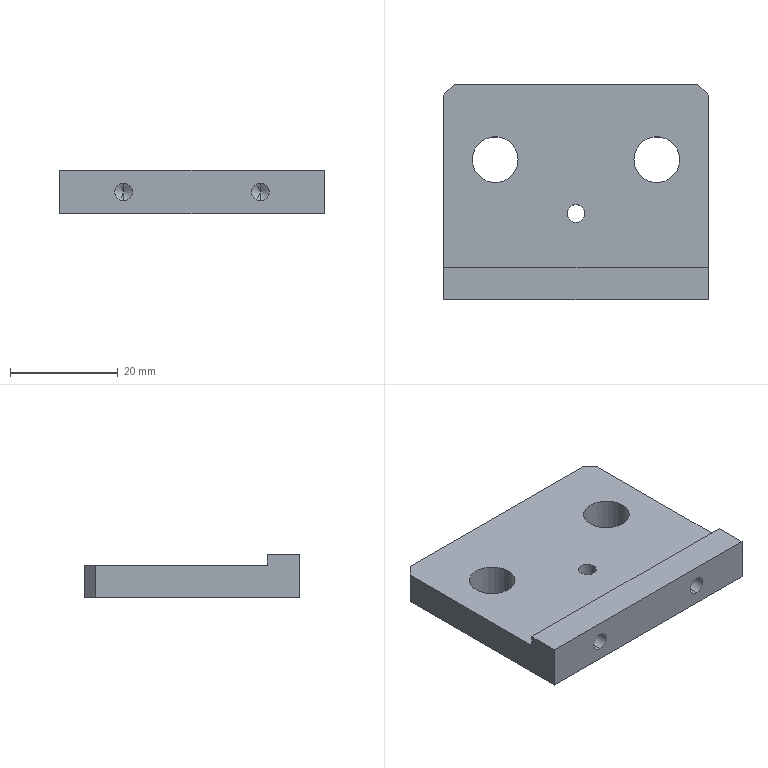Part | SolidWorks | features HoleWzd 2, ICE 2, Chamfer 1, Extrusion 1 | 1 solid | 24 faces | box 49.2 x 40 x 8 mm | volume 11464 mm3 | cylinder 10 | plane 10 | cone 4 | commonest cylinder face diameters 3.3 x6 8.5 x4
STEP:
#1=CARTESIAN_POINT('',(-1.65,-4.,0.));
#2=VERTEX_POINT('',#1);
#3=CARTESIAN_POINT('',(1.65,-4.,0.));
#4=VERTEX_POINT('',#3);
#5=CARTESIAN_POINT('',(0.,-4.,0.));
#6=DIRECTION('',(0.,0.,1.));
#7=DIRECTION('',(1.,0.,0.));
#8=AXIS2_PLACEMENT_3D('',#5,#6,#7);
#9=CIRCLE('',#8,1.65);
#10=EDGE_CURVE('',#2,#4,#9,.T.);
#11=ORIENTED_EDGE('',*,*,#10,.F.);
#12=CARTESIAN_POINT('',(-1.65,-4.,6.));
#13=VERTEX_POINT('',#12);
#14=CARTESIAN_POINT('',(-1.65,-4.,6.));
#15=DIRECTION('',(0.,0.,1.));
#16=VECTOR('',#15,1000.);
#17=LINE('',#14,#16);
#18=EDGE_CURVE('',#2,#13,#17,.T.);
#19=ORIENTED_EDGE('',*,*,#18,.T.);
#20=CARTESIAN_POINT('',(1.65,-4.,6.));
#21=VERTEX_POINT('',#20);
#22=CARTESIAN_POINT('',(0.,-4.,6.));
#23=DIRECTION('',(0.,0.,1.));
#24=DIRECTION('',(1.,0.,0.));
#25=AXIS2_PLACEMENT_3D('',#22,#23,#24);
#26=CIRCLE('',#25,1.65);
#27=EDGE_CURVE('',#13,#21,#26,.T.);
#28=ORIENTED_EDGE('',*,*,#27,.T.);
#29=CARTESIAN_POINT('',(1.65,-4.,6.));
#30=DIRECTION('',(0.,0.,1.));
#31=VECTOR('',#30,1000.);
#32=LINE('',#29,#31);
#33=EDGE_CURVE('',#4,#21,#32,.T.);
#34=ORIENTED_EDGE('',*,*,#33,.F.);
#35=EDGE_LOOP('',(#11,#19,#28,#34));
#36=FACE_OUTER_BOUND('',#35,.T.);
#37=CARTESIAN_POINT('',(0.,-4.,6.));
#38=DIRECTION('',(0.,0.,1.));
#39=DIRECTION('',(1.,0.,0.));
#40=AXIS2_PLACEMENT_3D('',#37,#38,#39);
#41=CYLINDRICAL_SURFACE('',#40,1.65);
#42=ADVANCED_FACE('',(#36),#41,.F.);
#43=CARTESIAN_POINT('',(-19.25,6.,6.));
#44=VERTEX_POINT('',#43);
#45=CARTESIAN_POINT('',(-10.75,6.,6.));
#46=VERTEX_POINT('',#45);
#47=CARTESIAN_POINT('',(-15.,6.,6.));
#48=DIRECTION('',(0.,0.,1.));
#49=DIRECTION('',(1.,0.,0.));
#50=AXIS2_PLACEMENT_3D('',#47,#48,#49);
#51=CIRCLE('',#50,4.25);
#52=EDGE_CURVE('',#44,#46,#51,.T.);
#53=ORIENTED_EDGE('',*,*,#52,.T.);
#54=CARTESIAN_POINT('',(-10.75,6.,0.));
#55=VERTEX_POINT('',#54);
#56=CARTESIAN_POINT('',(-10.75,6.,25.));
#57=DIRECTION('',(0.,0.,-1.));
#58=VECTOR('',#57,1000.);
#59=LINE('',#56,#58);
#60=EDGE_CURVE('',#46,#55,#59,.T.);
#61=ORIENTED_EDGE('',*,*,#60,.T.);
#62=CARTESIAN_POINT('',(-19.25,6.,0.));
#63=VERTEX_POINT('',#62);
#64=CARTESIAN_POINT('',(-15.,6.,0.));
#65=DIRECTION('',(0.,0.,-1.));
#66=DIRECTION('',(-1.,0.,0.));
#67=AXIS2_PLACEMENT_3D('',#64,#65,#66);
#68=CIRCLE('',#67,4.25);
#69=EDGE_CURVE('',#55,#63,#68,.T.);
#70=ORIENTED_EDGE('',*,*,#69,.T.);
#71=CARTESIAN_POINT('',(-19.25,6.,25.));
#72=DIRECTION('',(0.,0.,-1.));
#73=VECTOR('',#72,1000.);
#74=LINE('',#71,#73);
#75=EDGE_CURVE('',#44,#63,#74,.T.);
#76=ORIENTED_EDGE('',*,*,#75,.F.);
#77=EDGE_LOOP('',(#53,#61,#70,#76));
#78=FACE_OUTER_BOUND('',#77,.T.);
#79=CARTESIAN_POINT('',(-15.,6.,25.));
#80=DIRECTION('',(0.,0.,-1.));
#81=DIRECTION('',(-1.,0.,0.));
#82=AXIS2_PLACEMENT_3D('',#79,#80,#81);
#83=CYLINDRICAL_SURFACE('',#82,4.25);
#84=ADVANCED_FACE('',(#78),#83,.F.);
#85=CARTESIAN_POINT('',(10.75,6.,6.));
#86=VERTEX_POINT('',#85);
#87=CARTESIAN_POINT('',(19.25,6.,6.));
#88=VERTEX_POINT('',#87);
#89=CARTESIAN_POINT('',(15.,6.,6.));
#90=DIRECTION('',(0.,0.,1.));
#91=DIRECTION('',(1.,0.,0.));
#92=AXIS2_PLACEMENT_3D('',#89,#90,#91);
#93=CIRCLE('',#92,4.25);
#94=EDGE_CURVE('',#86,#88,#93,.T.);
#95=ORIENTED_EDGE('',*,*,#94,.T.);
#96=CARTESIAN_POINT('',(19.25,6.,0.));
#97=VERTEX_POINT('',#96);
#98=CARTESIAN_POINT('',(19.25,6.,25.));
#99=DIRECTION('',(0.,0.,-1.));
#100=VECTOR('',#99,1000.);
#101=LINE('',#98,#100);
#102=EDGE_CURVE('',#88,#97,#101,.T.);
#103=ORIENTED_EDGE('',*,*,#102,.T.);
#104=CARTESIAN_POINT('',(10.75,6.,0.));
#105=VERTEX_POINT('',#104);
#106=CARTESIAN_POINT('',(15.,6.,0.));
#107=DIRECTION('',(0.,0.,-1.));
#108=DIRECTION('',(-1.,0.,0.));
#109=AXIS2_PLACEMENT_3D('',#106,#107,#108);
#110=CIRCLE('',#109,4.25);
#111=EDGE_CURVE('',#97,#105,#110,.T.);
#112=ORIENTED_EDGE('',*,*,#111,.T.);
#113=CARTESIAN_POINT('',(10.75,6.,25.));
#114=DIRECTION('',(0.,0.,-1.));
#115=VECTOR('',#114,1000.);
#116=LINE('',#113,#115);
#117=EDGE_CURVE('',#86,#105,#116,.T.);
#118=ORIENTED_EDGE('',*,*,#117,.F.);
#119=EDGE_LOOP('',(#95,#103,#112,#118));
#120=FACE_OUTER_BOUND('',#119,.T.);
#121=CARTESIAN_POINT('',(15.,6.,25.));
#122=DIRECTION('',(0.,0.,-1.));
#123=DIRECTION('',(-1.,0.,0.));
#124=AXIS2_PLACEMENT_3D('',#121,#122,#123);
#125=CYLINDRICAL_SURFACE('',#124,4.25);
#126=ADVANCED_FACE('',(#120),#125,.F.);
#127=CARTESIAN_POINT('',(-12.7,-9.9,5.65));
#128=VERTEX_POINT('',#127);
#129=CARTESIAN_POINT('',(-12.7,-9.9,2.35));
#130=VERTEX_POINT('',#129);
#131=CARTESIAN_POINT('',(-12.7,-9.9,4.));
#132=DIRECTION('',(0.,-1.,0.));
#133=DIRECTION('',(0.,0.,-1.));
#134=AXIS2_PLACEMENT_3D('',#131,#132,#133);
#135=CIRCLE('',#134,1.65);
#136=EDGE_CURVE('',#128,#130,#135,.T.);
#137=ORIENTED_EDGE('',*,*,#136,.F.);
#138=CARTESIAN_POINT('',(-12.7,-20.,5.65));
#139=VERTEX_POINT('',#138);
#140=CARTESIAN_POINT('',(-12.7,-20.,5.65));
#141=DIRECTION('',(0.,-1.,0.));
#142=VECTOR('',#141,1000.);
#143=LINE('',#140,#142);
#144=EDGE_CURVE('',#128,#139,#143,.T.);
#145=ORIENTED_EDGE('',*,*,#144,.T.);
#146=CARTESIAN_POINT('',(-12.7,-20.,2.35));
#147=VERTEX_POINT('',#146);
#148=CARTESIAN_POINT('',(-12.7,-20.,4.));
#149=DIRECTION('',(0.,-1.,0.));
#150=DIRECTION('',(0.,0.,-1.));
#151=AXIS2_PLACEMENT_3D('',#148,#149,#150);
#152=CIRCLE('',#151,1.65);
#153=EDGE_CURVE('',#139,#147,#152,.T.);
#154=ORIENTED_EDGE('',*,*,#153,.T.);
#155=CARTESIAN_POINT('',(-12.7,-20.,2.35));
#156=DIRECTION('',(0.,-1.,0.));
#157=VECTOR('',#156,1000.);
#158=LINE('',#155,#157);
#159=EDGE_CURVE('',#130,#147,#158,.T.);
#160=ORIENTED_EDGE('',*,*,#159,.F.);
#161=EDGE_LOOP('',(#137,#145,#154,#160));
#162=FACE_OUTER_BOUND('',#161,.T.);
#163=CARTESIAN_POINT('',(-12.7,-20.,4.));
#164=DIRECTION('',(0.,-1.,0.));
#165=DIRECTION('',(0.,0.,-1.));
#166=AXIS2_PLACEMENT_3D('',#163,#164,#165);
#167=CYLINDRICAL_SURFACE('',#166,1.65);
#168=ADVANCED_FACE('',(#162),#167,.F.);
#169=CARTESIAN_POINT('',(-12.7,-8.909,4.));
#170=VERTEX_POINT('',#169);
#171=CARTESIAN_POINT('',(-12.7,-9.9,2.35));
#172=DIRECTION('',(0.,-0.515,-0.8572));
#173=VECTOR('',#172,1000.);
#174=LINE('',#171,#173);
#175=EDGE_CURVE('',#170,#130,#174,.T.);
#176=ORIENTED_EDGE('',*,*,#175,.F.);
#177=CARTESIAN_POINT('',(-12.7,-9.9,5.65));
#178=DIRECTION('',(0.,-0.515,0.8572));
#179=VECTOR('',#178,1000.);
#180=LINE('',#177,#179);
#181=EDGE_CURVE('',#170,#128,#180,.T.);
#182=ORIENTED_EDGE('',*,*,#181,.T.);
#183=ORIENTED_EDGE('',*,*,#136,.T.);
#184=EDGE_LOOP('',(#176,#182,#183));
#185=FACE_OUTER_BOUND('',#184,.T.);
#186=CARTESIAN_POINT('',(-12.7,-9.9,4.));
#187=DIRECTION('',(0.,-1.,0.));
#188=DIRECTION('',(0.,0.,-1.));
#189=AXIS2_PLACEMENT_3D('',#186,#187,#188);
#190=CONICAL_SURFACE('',#189,1.65,1.03);
#191=ADVANCED_FACE('',(#185),#190,.F.);
#192=CARTESIAN_POINT('',(12.7,-9.9,5.65));
#193=VERTEX_POINT('',#192);
#194=CARTESIAN_POINT('',(12.7,-9.9,2.35));
#195=VERTEX_POINT('',#194);
#196=CARTESIAN_POINT('',(12.7,-9.9,4.));
#197=DIRECTION('',(0.,-1.,0.));
#198=DIRECTION('',(0.,0.,-1.));
#199=AXIS2_PLACEMENT_3D('',#196,#197,#198);
#200=CIRCLE('',#199,1.65);
#201=EDGE_CURVE('',#193,#195,#200,.T.);
#202=ORIENTED_EDGE('',*,*,#201,.F.);
#203=CARTESIAN_POINT('',(12.7,-20.,5.65));
#204=VERTEX_POINT('',#203);
#205=CARTESIAN_POINT('',(12.7,-20.,5.65));
#206=DIRECTION('',(0.,-1.,0.));
#207=VECTOR('',#206,1000.);
#208=LINE('',#205,#207);
#209=EDGE_CURVE('',#193,#204,#208,.T.);
#210=ORIENTED_EDGE('',*,*,#209,.T.);
#211=CARTESIAN_POINT('',(12.7,-20.,2.35));
#212=VERTEX_POINT('',#211);
#213=CARTESIAN_POINT('',(12.7,-20.,4.));
#214=DIRECTION('',(0.,-1.,0.));
#215=DIRECTION('',(0.,0.,-1.));
#216=AXIS2_PLACEMENT_3D('',#213,#214,#215);
#217=CIRCLE('',#216,1.65);
#218=EDGE_CURVE('',#204,#212,#217,.T.);
#219=ORIENTED_EDGE('',*,*,#218,.T.);
#220=CARTESIAN_POINT('',(12.7,-20.,2.35));
#221=DIRECTION('',(0.,-1.,0.));
#222=VECTOR('',#221,1000.);
#223=LINE('',#220,#222);
#224=EDGE_CURVE('',#195,#212,#223,.T.);
#225=ORIENTED_EDGE('',*,*,#224,.F.);
#226=EDGE_LOOP('',(#202,#210,#219,#225));
#227=FACE_OUTER_BOUND('',#226,.T.);
#228=CARTESIAN_POINT('',(12.7,-20.,4.));
#229=DIRECTION('',(0.,-1.,0.));
#230=DIRECTION('',(0.,0.,-1.));
#231=AXIS2_PLACEMENT_3D('',#228,#229,#230);
#232=CYLINDRICAL_SURFACE('',#231,1.65);
#233=ADVANCED_FACE('',(#227),#232,.F.);
#234=CARTESIAN_POINT('',(12.7,-8.909,4.));
#235=VERTEX_POINT('',#234);
#236=CARTESIAN_POINT('',(12.7,-9.9,2.35));
#237=DIRECTION('',(0.,-0.515,-0.8572));
#238=VECTOR('',#237,1000.);
#239=LINE('',#236,#238);
#240=EDGE_CURVE('',#235,#195,#239,.T.);
#241=ORIENTED_EDGE('',*,*,#240,.F.);
#242=CARTESIAN_POINT('',(12.7,-9.9,5.65));
#243=DIRECTION('',(0.,-0.515,0.8572));
#244=VECTOR('',#243,1000.);
#245=LINE('',#242,#244);
#246=EDGE_CURVE('',#235,#193,#245,.T.);
#247=ORIENTED_EDGE('',*,*,#246,.T.);
#248=ORIENTED_EDGE('',*,*,#201,.T.);
#249=EDGE_LOOP('',(#241,#247,#248));
#250=FACE_OUTER_BOUND('',#249,.T.);
#251=CARTESIAN_POINT('',(12.7,-9.9,4.));
#252=DIRECTION('',(0.,-1.,0.));
#253=DIRECTION('',(0.,0.,-1.));
#254=AXIS2_PLACEMENT_3D('',#251,#252,#253);
#255=CONICAL_SURFACE('',#254,1.65,1.03);
#256=ADVANCED_FACE('',(#250),#255,.F.);
#257=CARTESIAN_POINT('',(22.6,20.,6.));
#258=VERTEX_POINT('',#257);
#259=CARTESIAN_POINT('',(-22.6,20.,6.));
#260=VERTEX_POINT('',#259);
#261=CARTESIAN_POINT('',(-24.6,20.,6.));
#262=DIRECTION('',(-1.,0.,0.));
#263=VECTOR('',#262,1000.);
#264=LINE('',#261,#263);
#265=EDGE_CURVE('',#258,#260,#264,.T.);
#266=ORIENTED_EDGE('',*,*,#265,.F.);
#267=CARTESIAN_POINT('',(22.6,20.,0.));
#268=VERTEX_POINT('',#267);
#269=CARTESIAN_POINT('',(22.6,20.,8.));
#270=DIRECTION('',(0.,0.,-1.));
#271=VECTOR('',#270,1000.);
#272=LINE('',#269,#271);
#273=EDGE_CURVE('',#258,#268,#272,.T.);
#274=ORIENTED_EDGE('',*,*,#273,.T.);
#275=CARTESIAN_POINT('',(-22.6,20.,0.));
#276=VERTEX_POINT('',#275);
#277=CARTESIAN_POINT('',(-24.6,20.,0.));
#278=DIRECTION('',(-1.,0.,0.));
#279=VECTOR('',#278,1000.);
#280=LINE('',#277,#279);
#281=EDGE_CURVE('',#268,#276,#280,.T.);
#282=ORIENTED_EDGE('',*,*,#281,.T.);
#283=CARTESIAN_POINT('',(-22.6,20.,8.));
#284=DIRECTION('',(0.,0.,1.));
#285=VECTOR('',#284,1000.);
#286=LINE('',#283,#285);
#287=EDGE_CURVE('',#276,#260,#286,.T.);
#288=ORIENTED_EDGE('',*,*,#287,.T.);
#289=EDGE_LOOP('',(#266,#274,#282,#288));
#290=FACE_OUTER_BOUND('',#289,.T.);
#291=CARTESIAN_POINT('',(-24.6,20.,8.));
#292=DIRECTION('',(0.,-1.,0.));
#293=DIRECTION('',(0.,0.,-1.));
#294=AXIS2_PLACEMENT_3D('',#291,#292,#293);
#295=PLANE('',#294);
#296=ADVANCED_FACE('',(#290),#295,.F.);
#297=ORIENTED_EDGE('',*,*,#273,.F.);
#298=CARTESIAN_POINT('',(24.6,18.,6.));
#299=VERTEX_POINT('',#298);
#300=CARTESIAN_POINT('',(22.6,20.,6.));
#301=DIRECTION('',(0.7071,-0.7071,0.));
#302=VECTOR('',#301,1000.);
#303=LINE('',#300,#302);
#304=EDGE_CURVE('',#258,#299,#303,.T.);
#305=ORIENTED_EDGE('',*,*,#304,.T.);
#306=CARTESIAN_POINT('',(24.6,18.,0.));
#307=VERTEX_POINT('',#306);
#308=CARTESIAN_POINT('',(24.6,18.,8.));
#309=DIRECTION('',(0.,0.,1.));
#310=VECTOR('',#309,1000.);
#311=LINE('',#308,#310);
#312=EDGE_CURVE('',#307,#299,#311,.T.);
#313=ORIENTED_EDGE('',*,*,#312,.F.);
#314=CARTESIAN_POINT('',(22.6,20.,0.));
#315=DIRECTION('',(0.7071,-0.7071,0.));
#316=VECTOR('',#315,1000.);
#317=LINE('',#314,#316);
#318=EDGE_CURVE('',#268,#307,#317,.T.);
#319=ORIENTED_EDGE('',*,*,#318,.F.);
#320=EDGE_LOOP('',(#297,#305,#313,#319));
#321=FACE_OUTER_BOUND('',#320,.T.);
#322=CARTESIAN_POINT('',(22.6,20.,8.));
#323=DIRECTION('',(-0.7071,-0.7071,0.));
#324=DIRECTION('',(0.,0.,-1.));
#325=AXIS2_PLACEMENT_3D('',#322,#323,#324);
#326=PLANE('',#325);
#327=ADVANCED_FACE('',(#321),#326,.F.);
#328=CARTESIAN_POINT('',(-24.6,18.,6.));
#329=VERTEX_POINT('',#328);
#330=CARTESIAN_POINT('',(-24.6,18.,0.));
#331=VERTEX_POINT('',#330);
#332=CARTESIAN_POINT('',(-24.6,18.,8.));
#333=DIRECTION('',(0.,0.,-1.));
#334=VECTOR('',#333,1000.);
#335=LINE('',#332,#334);
#336=EDGE_CURVE('',#329,#331,#335,.T.);
#337=ORIENTED_EDGE('',*,*,#336,.F.);
#338=CARTESIAN_POINT('',(-24.6,18.,6.));
#339=DIRECTION('',(0.7071,0.7071,0.));
#340=VECTOR('',#339,1000.);
#341=LINE('',#338,#340);
#342=EDGE_CURVE('',#329,#260,#341,.T.);
#343=ORIENTED_EDGE('',*,*,#342,.T.);
#344=ORIENTED_EDGE('',*,*,#287,.F.);
#345=CARTESIAN_POINT('',(-24.6,18.,0.));
#346=DIRECTION('',(0.7071,0.7071,0.));
#347=VECTOR('',#346,1000.);
#348=LINE('',#345,#347);
#349=EDGE_CURVE('',#331,#276,#348,.T.);
#350=ORIENTED_EDGE('',*,*,#349,.F.);
#351=EDGE_LOOP('',(#337,#343,#344,#350));
#352=FACE_OUTER_BOUND('',#351,.T.);
#353=CARTESIAN_POINT('',(-24.6,18.,8.));
#354=DIRECTION('',(0.7071,-0.7071,0.));
#355=DIRECTION('',(0.,0.,-1.));
#356=AXIS2_PLACEMENT_3D('',#353,#354,#355);
#357=PLANE('',#356);
#358=ADVANCED_FACE('',(#352),#357,.F.);
#359=CARTESIAN_POINT('',(24.6,-14.,6.));
#360=VERTEX_POINT('',#359);
#361=CARTESIAN_POINT('',(24.6,20.,6.));
#362=DIRECTION('',(0.,1.,0.));
#363=VECTOR('',#362,1000.);
#364=LINE('',#361,#363);
#365=EDGE_CURVE('',#360,#299,#364,.T.);
#366=ORIENTED_EDGE('',*,*,#365,.F.);
#367=CARTESIAN_POINT('',(24.6,-14.,8.));
#368=VERTEX_POINT('',#367);
#369=CARTESIAN_POINT('',(24.6,-14.,8.));
#370=DIRECTION('',(0.,0.,1.));
#371=VECTOR('',#370,1000.);
#372=LINE('',#369,#371);
#373=EDGE_CURVE('',#360,#368,#372,.T.);
#374=ORIENTED_EDGE('',*,*,#373,.T.);
#375=CARTESIAN_POINT('',(24.6,-20.,8.));
#376=VERTEX_POINT('',#375);
#377=CARTESIAN_POINT('',(24.6,20.,8.));
#378=DIRECTION('',(0.,1.,0.));
#379=VECTOR('',#378,1000.);
#380=LINE('',#377,#379);
#381=EDGE_CURVE('',#376,#368,#380,.T.);
#382=ORIENTED_EDGE('',*,*,#381,.F.);
#383=CARTESIAN_POINT('',(24.6,-20.,0.));
#384=VERTEX_POINT('',#383);
#385=CARTESIAN_POINT('',(24.6,-20.,8.));
#386=DIRECTION('',(0.,0.,-1.));
#387=VECTOR('',#386,1000.);
#388=LINE('',#385,#387);
#389=EDGE_CURVE('',#376,#384,#388,.T.);
#390=ORIENTED_EDGE('',*,*,#389,.T.);
#391=CARTESIAN_POINT('',(24.6,20.,0.));
#392=DIRECTION('',(0.,1.,0.));
#393=VECTOR('',#392,1000.);
#394=LINE('',#391,#393);
#395=EDGE_CURVE('',#384,#307,#394,.T.);
#396=ORIENTED_EDGE('',*,*,#395,.T.);
#397=ORIENTED_EDGE('',*,*,#312,.T.);
#398=EDGE_LOOP('',(#366,#374,#382,#390,#396,#397));
#399=FACE_OUTER_BOUND('',#398,.T.);
#400=CARTESIAN_POINT('',(24.6,20.,8.));
#401=DIRECTION('',(-1.,0.,0.));
#402=DIRECTION('',(0.,-1.,0.));
#403=AXIS2_PLACEMENT_3D('',#400,#401,#402);
#404=PLANE('',#403);
#405=ADVANCED_FACE('',(#399),#404,.F.);
#406=CARTESIAN_POINT('',(-24.6,-14.,8.));
#407=VERTEX_POINT('',#406);
#408=CARTESIAN_POINT('',(-24.6,-20.,8.));
#409=VERTEX_POINT('',#408);
#410=CARTESIAN_POINT('',(-24.6,20.,8.));
#411=DIRECTION('',(0.,-1.,0.));
#412=VECTOR('',#411,1000.);
#413=LINE('',#410,#412);
#414=EDGE_CURVE('',#407,#409,#413,.T.);
#415=ORIENTED_EDGE('',*,*,#414,.F.);
#416=CARTESIAN_POINT('',(-24.6,-14.,6.));
#417=VERTEX_POINT('',#416);
#418=CARTESIAN_POINT('',(-24.6,-14.,8.));
#419=DIRECTION('',(0.,0.,-1.));
#420=VECTOR('',#419,1000.);
#421=LINE('',#418,#420);
#422=EDGE_CURVE('',#407,#417,#421,.T.);
#423=ORIENTED_EDGE('',*,*,#422,.T.);
#424=CARTESIAN_POINT('',(-24.6,20.,6.));
#425=DIRECTION('',(0.,-1.,0.));
#426=VECTOR('',#425,1000.);
#427=LINE('',#424,#426);
#428=EDGE_CURVE('',#329,#417,#427,.T.);
#429=ORIENTED_EDGE('',*,*,#428,.F.);
#430=ORIENTED_EDGE('',*,*,#336,.T.);
#431=CARTESIAN_POINT('',(-24.6,-20.,0.));
#432=VERTEX_POINT('',#431);
#433=CARTESIAN_POINT('',(-24.6,20.,0.));
#434=DIRECTION('',(0.,-1.,0.));
#435=VECTOR('',#434,1000.);
#436=LINE('',#433,#435);
#437=EDGE_CURVE('',#331,#432,#436,.T.);
#438=ORIENTED_EDGE('',*,*,#437,.T.);
#439=CARTESIAN_POINT('',(-24.6,-20.,8.));
#440=DIRECTION('',(0.,0.,-1.));
#441=VECTOR('',#440,1000.);
#442=LINE('',#439,#441);
#443=EDGE_CURVE('',#409,#432,#442,.T.);
#444=ORIENTED_EDGE('',*,*,#443,.F.);
#445=EDGE_LOOP('',(#415,#423,#429,#430,#438,#444));
#446=FACE_OUTER_BOUND('',#445,.T.);
#447=CARTESIAN_POINT('',(-24.6,20.,8.));
#448=DIRECTION('',(1.,0.,0.));
#449=DIRECTION('',(0.,1.,0.));
#450=AXIS2_PLACEMENT_3D('',#447,#448,#449);
#451=PLANE('',#450);
#452=ADVANCED_FACE('',(#446),#451,.F.);
#453=CARTESIAN_POINT('',(-12.7,-20.,4.));
#454=DIRECTION('',(0.,-1.,0.));
#455=DIRECTION('',(0.,0.,-1.));
#456=AXIS2_PLACEMENT_3D('',#453,#454,#455);
#457=CIRCLE('',#456,1.65);
#458=EDGE_CURVE('',#147,#139,#457,.T.);
#459=ORIENTED_EDGE('',*,*,#458,.F.);
#460=ORIENTED_EDGE('',*,*,#153,.F.);
#461=EDGE_LOOP('',(#459,#460));
#462=FACE_BOUND('',#461,.T.);
#463=CARTESIAN_POINT('',(12.7,-20.,4.));
#464=DIRECTION('',(0.,-1.,0.));
#465=DIRECTION('',(0.,0.,-1.));
#466=AXIS2_PLACEMENT_3D('',#463,#464,#465);
#467=CIRCLE('',#466,1.65);
#468=EDGE_CURVE('',#212,#204,#467,.T.);
#469=ORIENTED_EDGE('',*,*,#468,.F.);
#470=ORIENTED_EDGE('',*,*,#218,.F.);
#471=EDGE_LOOP('',(#469,#470));
#472=FACE_BOUND('',#471,.T.);
#473=CARTESIAN_POINT('',(-24.6,-20.,0.));
#474=DIRECTION('',(1.,0.,0.));
#475=VECTOR('',#474,1000.);
#476=LINE('',#473,#475);
#477=EDGE_CURVE('',#432,#384,#476,.T.);
#478=ORIENTED_EDGE('',*,*,#477,.T.);
#479=ORIENTED_EDGE('',*,*,#389,.F.);
#480=CARTESIAN_POINT('',(-24.6,-20.,8.));
#481=DIRECTION('',(1.,0.,0.));
#482=VECTOR('',#481,1000.);
#483=LINE('',#480,#482);
#484=EDGE_CURVE('',#409,#376,#483,.T.);
#485=ORIENTED_EDGE('',*,*,#484,.F.);
#486=ORIENTED_EDGE('',*,*,#443,.T.);
#487=EDGE_LOOP('',(#478,#479,#485,#486));
#488=FACE_OUTER_BOUND('',#487,.T.);
#489=CARTESIAN_POINT('',(-24.6,-20.,8.));
#490=DIRECTION('',(0.,1.,0.));
#491=DIRECTION('',(0.,0.,1.));
#492=AXIS2_PLACEMENT_3D('',#489,#490,#491);
#493=PLANE('',#492);
#494=ADVANCED_FACE('',(#462,#472,#488),#493,.F.);
#495=CARTESIAN_POINT('',(-24.969,-14.,8.));
#496=DIRECTION('',(1.,0.,0.));
#497=VECTOR('',#496,1000.);
#498=LINE('',#495,#497);
#499=EDGE_CURVE('',#407,#368,#498,.T.);
#500=ORIENTED_EDGE('',*,*,#499,.F.);
#501=ORIENTED_EDGE('',*,*,#414,.T.);
#502=ORIENTED_EDGE('',*,*,#484,.T.);
#503=ORIENTED_EDGE('',*,*,#381,.T.);
#504=EDGE_LOOP('',(#500,#501,#502,#503));
#505=FACE_OUTER_BOUND('',#504,.T.);
#506=CARTESIAN_POINT('',(0.,0.,8.));
#507=DIRECTION('',(0.,0.,1.));
#508=DIRECTION('',(1.,0.,0.));
#509=AXIS2_PLACEMENT_3D('',#506,#507,#508);
#510=PLANE('',#509);
#511=ADVANCED_FACE('',(#505),#510,.T.);
#512=CARTESIAN_POINT('',(0.,-4.,0.));
#513=DIRECTION('',(0.,0.,1.));
#514=DIRECTION('',(1.,0.,0.));
#515=AXIS2_PLACEMENT_3D('',#512,#513,#514);
#516=CIRCLE('',#515,1.65);
#517=EDGE_CURVE('',#4,#2,#516,.T.);
#518=ORIENTED_EDGE('',*,*,#517,.T.);
#519=ORIENTED_EDGE('',*,*,#10,.T.);
#520=EDGE_LOOP('',(#518,#519));
#521=FACE_BOUND('',#520,.T.);
#522=CARTESIAN_POINT('',(-15.,6.,0.));
#523=DIRECTION('',(0.,0.,-1.));
#524=DIRECTION('',(-1.,0.,0.));
#525=AXIS2_PLACEMENT_3D('',#522,#523,#524);
#526=CIRCLE('',#525,4.25);
#527=EDGE_CURVE('',#63,#55,#526,.T.);
#528=ORIENTED_EDGE('',*,*,#527,.F.);
#529=ORIENTED_EDGE('',*,*,#69,.F.);
#530=EDGE_LOOP('',(#528,#529));
#531=FACE_BOUND('',#530,.T.);
#532=CARTESIAN_POINT('',(15.,6.,0.));
#533=DIRECTION('',(0.,0.,-1.));
#534=DIRECTION('',(-1.,0.,0.));
#535=AXIS2_PLACEMENT_3D('',#532,#533,#534);
#536=CIRCLE('',#535,4.25);
#537=EDGE_CURVE('',#105,#97,#536,.T.);
#538=ORIENTED_EDGE('',*,*,#537,.F.);
#539=ORIENTED_EDGE('',*,*,#111,.F.);
#540=EDGE_LOOP('',(#538,#539));
#541=FACE_BOUND('',#540,.T.);
#542=ORIENTED_EDGE('',*,*,#281,.F.);
#543=ORIENTED_EDGE('',*,*,#318,.T.);
#544=ORIENTED_EDGE('',*,*,#395,.F.);
#545=ORIENTED_EDGE('',*,*,#477,.F.);
#546=ORIENTED_EDGE('',*,*,#437,.F.);
#547=ORIENTED_EDGE('',*,*,#349,.T.);
#548=EDGE_LOOP('',(#542,#543,#544,#545,#546,#547));
#549=FACE_OUTER_BOUND('',#548,.T.);
#550=CARTESIAN_POINT('',(0.,0.,0.));
#551=DIRECTION('',(0.,0.,1.));
#552=DIRECTION('',(1.,0.,0.));
#553=AXIS2_PLACEMENT_3D('',#550,#551,#552);
#554=PLANE('',#553);
#555=ADVANCED_FACE('',(#521,#531,#541,#549),#554,.F.);
#556=ORIENTED_EDGE('',*,*,#246,.F.);
#557=ORIENTED_EDGE('',*,*,#240,.T.);
#558=CARTESIAN_POINT('',(12.7,-9.9,4.));
#559=DIRECTION('',(0.,-1.,0.));
#560=DIRECTION('',(0.,0.,-1.));
#561=AXIS2_PLACEMENT_3D('',#558,#559,#560);
#562=CIRCLE('',#561,1.65);
#563=EDGE_CURVE('',#195,#193,#562,.T.);
#564=ORIENTED_EDGE('',*,*,#563,.T.);
#565=EDGE_LOOP('',(#556,#557,#564));
#566=FACE_OUTER_BOUND('',#565,.T.);
#567=CARTESIAN_POINT('',(12.7,-9.9,4.));
#568=DIRECTION('',(0.,-1.,0.));
#569=DIRECTION('',(0.,0.,-1.));
#570=AXIS2_PLACEMENT_3D('',#567,#568,#569);
#571=CONICAL_SURFACE('',#570,1.65,1.03);
#572=ADVANCED_FACE('',(#566),#571,.F.);
#573=ORIENTED_EDGE('',*,*,#209,.F.);
#574=ORIENTED_EDGE('',*,*,#563,.F.);
#575=ORIENTED_EDGE('',*,*,#224,.T.);
#576=ORIENTED_EDGE('',*,*,#468,.T.);
#577=EDGE_LOOP('',(#573,#574,#575,#576));
#578=FACE_OUTER_BOUND('',#577,.T.);
#579=CARTESIAN_POINT('',(12.7,-20.,4.));
#580=DIRECTION('',(0.,-1.,0.));
#581=DIRECTION('',(0.,0.,-1.));
#582=AXIS2_PLACEMENT_3D('',#579,#580,#581);
#583=CYLINDRICAL_SURFACE('',#582,1.65);
#584=ADVANCED_FACE('',(#578),#583,.F.);
#585=ORIENTED_EDGE('',*,*,#181,.F.);
#586=ORIENTED_EDGE('',*,*,#175,.T.);
#587=CARTESIAN_POINT('',(-12.7,-9.9,4.));
#588=DIRECTION('',(0.,-1.,0.));
#589=DIRECTION('',(0.,0.,-1.));
#590=AXIS2_PLACEMENT_3D('',#587,#588,#589);
#591=CIRCLE('',#590,1.65);
#592=EDGE_CURVE('',#130,#128,#591,.T.);
#593=ORIENTED_EDGE('',*,*,#592,.T.);
#594=EDGE_LOOP('',(#585,#586,#593));
#595=FACE_OUTER_BOUND('',#594,.T.);
#596=CARTESIAN_POINT('',(-12.7,-9.9,4.));
#597=DIRECTION('',(0.,-1.,0.));
#598=DIRECTION('',(0.,0.,-1.));
#599=AXIS2_PLACEMENT_3D('',#596,#597,#598);
#600=CONICAL_SURFACE('',#599,1.65,1.03);
#601=ADVANCED_FACE('',(#595),#600,.F.);
#602=ORIENTED_EDGE('',*,*,#144,.F.);
#603=ORIENTED_EDGE('',*,*,#592,.F.);
#604=ORIENTED_EDGE('',*,*,#159,.T.);
#605=ORIENTED_EDGE('',*,*,#458,.T.);
#606=EDGE_LOOP('',(#602,#603,#604,#605));
#607=FACE_OUTER_BOUND('',#606,.T.);
#608=CARTESIAN_POINT('',(-12.7,-20.,4.));
#609=DIRECTION('',(0.,-1.,0.));
#610=DIRECTION('',(0.,0.,-1.));
#611=AXIS2_PLACEMENT_3D('',#608,#609,#610);
#612=CYLINDRICAL_SURFACE('',#611,1.65);
#613=ADVANCED_FACE('',(#607),#612,.F.);
#614=CARTESIAN_POINT('',(-24.969,-14.,6.));
#615=DIRECTION('',(1.,0.,0.));
#616=VECTOR('',#615,1000.);
#617=LINE('',#614,#616);
#618=EDGE_CURVE('',#417,#360,#617,.T.);
#619=ORIENTED_EDGE('',*,*,#618,.F.);
#620=ORIENTED_EDGE('',*,*,#422,.F.);
#621=ORIENTED_EDGE('',*,*,#499,.T.);
#622=ORIENTED_EDGE('',*,*,#373,.F.);
#623=EDGE_LOOP('',(#619,#620,#621,#622));
#624=FACE_OUTER_BOUND('',#623,.T.);
#625=CARTESIAN_POINT('',(-24.969,-14.,6.));
#626=DIRECTION('',(0.,-1.,0.));
#627=DIRECTION('',(0.,0.,-1.));
#628=AXIS2_PLACEMENT_3D('',#625,#626,#627);
#629=PLANE('',#628);
#630=ADVANCED_FACE('',(#624),#629,.F.);
#631=CARTESIAN_POINT('',(0.,-4.,6.));
#632=DIRECTION('',(0.,0.,1.));
#633=DIRECTION('',(1.,0.,0.));
#634=AXIS2_PLACEMENT_3D('',#631,#632,#633);
#635=CIRCLE('',#634,1.65);
#636=EDGE_CURVE('',#21,#13,#635,.T.);
#637=ORIENTED_EDGE('',*,*,#636,.F.);
#638=ORIENTED_EDGE('',*,*,#27,.F.);
#639=EDGE_LOOP('',(#637,#638));
#640=FACE_BOUND('',#639,.T.);
#641=ORIENTED_EDGE('',*,*,#52,.F.);
#642=CARTESIAN_POINT('',(-15.,6.,6.));
#643=DIRECTION('',(0.,0.,1.));
#644=DIRECTION('',(1.,0.,0.));
#645=AXIS2_PLACEMENT_3D('',#642,#643,#644);
#646=CIRCLE('',#645,4.25);
#647=EDGE_CURVE('',#46,#44,#646,.T.);
#648=ORIENTED_EDGE('',*,*,#647,.F.);
#649=EDGE_LOOP('',(#641,#648));
#650=FACE_BOUND('',#649,.T.);
#651=ORIENTED_EDGE('',*,*,#94,.F.);
#652=CARTESIAN_POINT('',(15.,6.,6.));
#653=DIRECTION('',(0.,0.,1.));
#654=DIRECTION('',(1.,0.,0.));
#655=AXIS2_PLACEMENT_3D('',#652,#653,#654);
#656=CIRCLE('',#655,4.25);
#657=EDGE_CURVE('',#88,#86,#656,.T.);
#658=ORIENTED_EDGE('',*,*,#657,.F.);
#659=EDGE_LOOP('',(#651,#658));
#660=FACE_BOUND('',#659,.T.);
#661=ORIENTED_EDGE('',*,*,#365,.T.);
#662=ORIENTED_EDGE('',*,*,#304,.F.);
#663=ORIENTED_EDGE('',*,*,#265,.T.);
#664=ORIENTED_EDGE('',*,*,#342,.F.);
#665=ORIENTED_EDGE('',*,*,#428,.T.);
#666=ORIENTED_EDGE('',*,*,#618,.T.);
#667=EDGE_LOOP('',(#661,#662,#663,#664,#665,#666));
#668=FACE_OUTER_BOUND('',#667,.T.);
#669=CARTESIAN_POINT('',(0.,0.,6.));
#670=DIRECTION('',(0.,0.,1.));
#671=DIRECTION('',(1.,0.,0.));
#672=AXIS2_PLACEMENT_3D('',#669,#670,#671);
#673=PLANE('',#672);
#674=ADVANCED_FACE('',(#640,#650,#660,#668),#673,.T.);
#675=ORIENTED_EDGE('',*,*,#102,.F.);
#676=ORIENTED_EDGE('',*,*,#657,.T.);
#677=ORIENTED_EDGE('',*,*,#117,.T.);
#678=ORIENTED_EDGE('',*,*,#537,.T.);
#679=EDGE_LOOP('',(#675,#676,#677,#678));
#680=FACE_OUTER_BOUND('',#679,.T.);
#681=CARTESIAN_POINT('',(15.,6.,25.));
#682=DIRECTION('',(0.,0.,-1.));
#683=DIRECTION('',(-1.,0.,0.));
#684=AXIS2_PLACEMENT_3D('',#681,#682,#683);
#685=CYLINDRICAL_SURFACE('',#684,4.25);
#686=ADVANCED_FACE('',(#680),#685,.F.);
#687=ORIENTED_EDGE('',*,*,#60,.F.);
#688=ORIENTED_EDGE('',*,*,#647,.T.);
#689=ORIENTED_EDGE('',*,*,#75,.T.);
#690=ORIENTED_EDGE('',*,*,#527,.T.);
#691=EDGE_LOOP('',(#687,#688,#689,#690));
#692=FACE_OUTER_BOUND('',#691,.T.);
#693=CARTESIAN_POINT('',(-15.,6.,25.));
#694=DIRECTION('',(0.,0.,-1.));
#695=DIRECTION('',(-1.,0.,0.));
#696=AXIS2_PLACEMENT_3D('',#693,#694,#695);
#697=CYLINDRICAL_SURFACE('',#696,4.25);
#698=ADVANCED_FACE('',(#692),#697,.F.);
#699=ORIENTED_EDGE('',*,*,#18,.F.);
#700=ORIENTED_EDGE('',*,*,#517,.F.);
#701=ORIENTED_EDGE('',*,*,#33,.T.);
#702=ORIENTED_EDGE('',*,*,#636,.T.);
#703=EDGE_LOOP('',(#699,#700,#701,#702));
#704=FACE_OUTER_BOUND('',#703,.T.);
#705=CARTESIAN_POINT('',(0.,-4.,6.));
#706=DIRECTION('',(0.,0.,1.));
#707=DIRECTION('',(1.,0.,0.));
#708=AXIS2_PLACEMENT_3D('',#705,#706,#707);
#709=CYLINDRICAL_SURFACE('',#708,1.65);
#710=ADVANCED_FACE('',(#704),#709,.F.);
#711=CLOSED_SHELL('',(#42,#84,#126,#168,#191,#233,#256,#296,#327,#358,#405,#452,#494,#511,#555,#572,#584,#601,#613,#630,#674,#686,#698,#710));
#712=MANIFOLD_SOLID_BREP('',#711);
#713=CARTESIAN_POINT('',(0.,0.,0.));
#714=DIRECTION('',(0.,0.,1.));
#715=DIRECTION('',(1.,0.,0.));
#716=AXIS2_PLACEMENT_3D('',#713,#714,#715);
#717=(LENGTH_UNIT()NAMED_UNIT(*)SI_UNIT(.MILLI.,.METRE.));
#718=UNCERTAINTY_MEASURE_WITH_UNIT(LENGTH_MEASURE(0.00001),#717,'','');
#719=(NAMED_UNIT(*)PLANE_ANGLE_UNIT()SI_UNIT($,.RADIAN.));
#720=(NAMED_UNIT(*)SI_UNIT($,.STERADIAN.)SOLID_ANGLE_UNIT());
#721=(GEOMETRIC_REPRESENTATION_CONTEXT(3)GLOBAL_UNCERTAINTY_ASSIGNED_CONTEXT((#718))GLOBAL_UNIT_ASSIGNED_CONTEXT((#717,#719,#720))REPRESENTATION_CONTEXT('',''));
#722=ADVANCED_BREP_SHAPE_REPRESENTATION('',(#712,#716),#721);